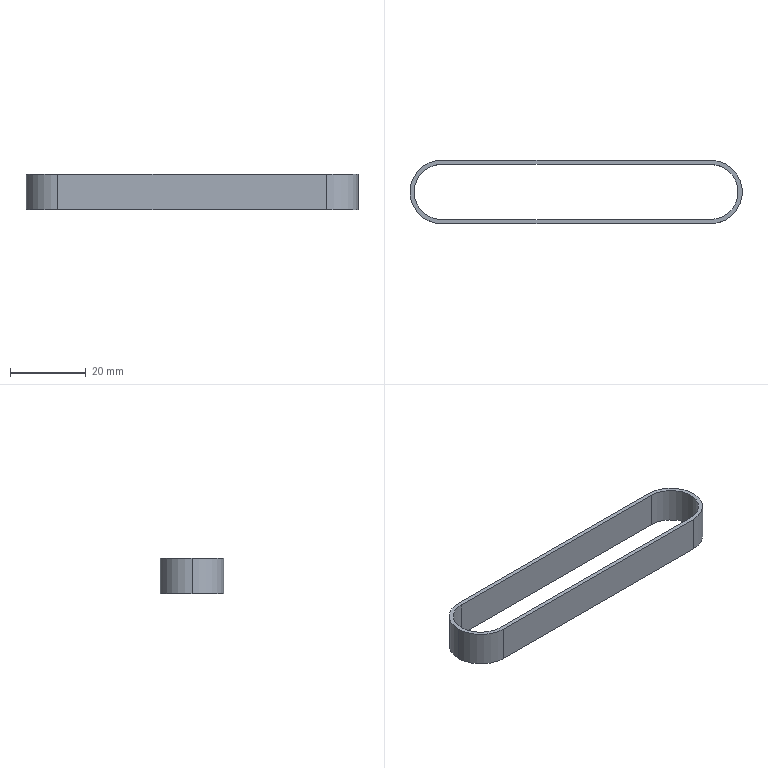Part | NX | features BREP 1 | 1 solid | 12 faces | box 87.76 x 16.76 x 9.5 mm | volume 1998 mm3 | plane 6 | cylinder 6 | commonest cylinder face diameters 14.56 x3 16.76 x3
STEP:
#1=CARTESIAN_POINT('',(-71.,-7.28,-4.75));
#2=VERTEX_POINT('',#1);
#3=CARTESIAN_POINT('',(0.,-7.28,-4.75));
#4=VERTEX_POINT('',#3);
#5=CARTESIAN_POINT('',(0.,-7.28,-4.75));
#6=DIRECTION('',(1.,0.,0.));
#7=VECTOR('',#6,1000.);
#8=LINE('',#5,#7);
#9=EDGE_CURVE('',#2,#4,#8,.T.);
#10=ORIENTED_EDGE('',*,*,#9,.F.);
#11=CARTESIAN_POINT('',(-71.,-7.28,4.75));
#12=VERTEX_POINT('',#11);
#13=CARTESIAN_POINT('',(-71.,-7.28,4.75));
#14=DIRECTION('',(0.,0.,-1.));
#15=VECTOR('',#14,1000.);
#16=LINE('',#13,#15);
#17=EDGE_CURVE('',#12,#2,#16,.T.);
#18=ORIENTED_EDGE('',*,*,#17,.F.);
#19=CARTESIAN_POINT('',(0.,-7.28,4.75));
#20=VERTEX_POINT('',#19);
#21=CARTESIAN_POINT('',(0.,-7.28,4.75));
#22=DIRECTION('',(1.,0.,0.));
#23=VECTOR('',#22,1000.);
#24=LINE('',#21,#23);
#25=EDGE_CURVE('',#12,#20,#24,.T.);
#26=ORIENTED_EDGE('',*,*,#25,.T.);
#27=CARTESIAN_POINT('',(0.,-7.28,4.75));
#28=DIRECTION('',(0.,0.,-1.));
#29=VECTOR('',#28,1000.);
#30=LINE('',#27,#29);
#31=EDGE_CURVE('',#20,#4,#30,.T.);
#32=ORIENTED_EDGE('',*,*,#31,.T.);
#33=EDGE_LOOP('',(#10,#18,#26,#32));
#34=FACE_BOUND('',#33,.T.);
#35=CARTESIAN_POINT('',(0.,-7.28,4.75));
#36=DIRECTION('',(0.,1.,0.));
#37=DIRECTION('',(0.,0.,1.));
#38=AXIS2_PLACEMENT_3D('',#35,#36,#37);
#39=PLANE('',#38);
#40=ADVANCED_FACE('',(#34),#39,.T.);
#41=CARTESIAN_POINT('',(-78.28,0.,4.75));
#42=VERTEX_POINT('',#41);
#43=CARTESIAN_POINT('',(-78.28,0.,-4.75));
#44=VERTEX_POINT('',#43);
#45=CARTESIAN_POINT('',(-78.28,0.,4.75));
#46=DIRECTION('',(0.,0.,-1.));
#47=VECTOR('',#46,1000.);
#48=LINE('',#45,#47);
#49=EDGE_CURVE('',#42,#44,#48,.T.);
#50=ORIENTED_EDGE('',*,*,#49,.F.);
#51=CARTESIAN_POINT('',(-71.,0.,4.75));
#52=DIRECTION('',(0.,0.,1.));
#53=DIRECTION('',(-1.,0.,0.));
#54=AXIS2_PLACEMENT_3D('',#51,#52,#53);
#55=CIRCLE('',#54,7.28);
#56=EDGE_CURVE('',#42,#12,#55,.T.);
#57=ORIENTED_EDGE('',*,*,#56,.T.);
#58=ORIENTED_EDGE('',*,*,#17,.T.);
#59=CARTESIAN_POINT('',(-71.,0.,-4.75));
#60=DIRECTION('',(0.,0.,1.));
#61=DIRECTION('',(-1.,0.,0.));
#62=AXIS2_PLACEMENT_3D('',#59,#60,#61);
#63=CIRCLE('',#62,7.28);
#64=EDGE_CURVE('',#44,#2,#63,.T.);
#65=ORIENTED_EDGE('',*,*,#64,.F.);
#66=EDGE_LOOP('',(#50,#57,#58,#65));
#67=FACE_BOUND('',#66,.T.);
#68=CARTESIAN_POINT('',(-71.,0.,4.75));
#69=DIRECTION('',(0.,0.,-1.));
#70=DIRECTION('',(-1.,0.,0.));
#71=AXIS2_PLACEMENT_3D('',#68,#69,#70);
#72=CYLINDRICAL_SURFACE('',#71,7.28);
#73=ADVANCED_FACE('',(#67),#72,.F.);
#74=CARTESIAN_POINT('',(0.,7.28,-4.75));
#75=VERTEX_POINT('',#74);
#76=CARTESIAN_POINT('',(-71.,7.28,-4.75));
#77=VERTEX_POINT('',#76);
#78=CARTESIAN_POINT('',(0.,7.28,-4.75));
#79=DIRECTION('',(-1.,0.,0.));
#80=VECTOR('',#79,1000.);
#81=LINE('',#78,#80);
#82=EDGE_CURVE('',#75,#77,#81,.T.);
#83=ORIENTED_EDGE('',*,*,#82,.F.);
#84=CARTESIAN_POINT('',(0.,7.28,4.75));
#85=VERTEX_POINT('',#84);
#86=CARTESIAN_POINT('',(0.,7.28,4.75));
#87=DIRECTION('',(0.,0.,-1.));
#88=VECTOR('',#87,1000.);
#89=LINE('',#86,#88);
#90=EDGE_CURVE('',#85,#75,#89,.T.);
#91=ORIENTED_EDGE('',*,*,#90,.F.);
#92=CARTESIAN_POINT('',(-71.,7.28,4.75));
#93=VERTEX_POINT('',#92);
#94=CARTESIAN_POINT('',(0.,7.28,4.75));
#95=DIRECTION('',(-1.,0.,0.));
#96=VECTOR('',#95,1000.);
#97=LINE('',#94,#96);
#98=EDGE_CURVE('',#85,#93,#97,.T.);
#99=ORIENTED_EDGE('',*,*,#98,.T.);
#100=CARTESIAN_POINT('',(-71.,7.28,4.75));
#101=DIRECTION('',(0.,0.,-1.));
#102=VECTOR('',#101,1000.);
#103=LINE('',#100,#102);
#104=EDGE_CURVE('',#93,#77,#103,.T.);
#105=ORIENTED_EDGE('',*,*,#104,.T.);
#106=EDGE_LOOP('',(#83,#91,#99,#105));
#107=FACE_BOUND('',#106,.T.);
#108=CARTESIAN_POINT('',(0.,7.28,4.75));
#109=DIRECTION('',(0.,-1.,0.));
#110=DIRECTION('',(0.,0.,-1.));
#111=AXIS2_PLACEMENT_3D('',#108,#109,#110);
#112=PLANE('',#111);
#113=ADVANCED_FACE('',(#107),#112,.T.);
#114=CARTESIAN_POINT('',(0.,0.,-4.75));
#115=DIRECTION('',(0.,0.,1.));
#116=DIRECTION('',(-1.,0.,0.));
#117=AXIS2_PLACEMENT_3D('',#114,#115,#116);
#118=CIRCLE('',#117,7.28);
#119=EDGE_CURVE('',#4,#75,#118,.T.);
#120=ORIENTED_EDGE('',*,*,#119,.F.);
#121=ORIENTED_EDGE('',*,*,#31,.F.);
#122=CARTESIAN_POINT('',(0.,0.,4.75));
#123=DIRECTION('',(0.,0.,1.));
#124=DIRECTION('',(-1.,0.,0.));
#125=AXIS2_PLACEMENT_3D('',#122,#123,#124);
#126=CIRCLE('',#125,7.28);
#127=EDGE_CURVE('',#20,#85,#126,.T.);
#128=ORIENTED_EDGE('',*,*,#127,.T.);
#129=ORIENTED_EDGE('',*,*,#90,.T.);
#130=EDGE_LOOP('',(#120,#121,#128,#129));
#131=FACE_BOUND('',#130,.T.);
#132=CARTESIAN_POINT('',(0.,0.,4.75));
#133=DIRECTION('',(0.,0.,-1.));
#134=DIRECTION('',(-1.,0.,0.));
#135=AXIS2_PLACEMENT_3D('',#132,#133,#134);
#136=CYLINDRICAL_SURFACE('',#135,7.28);
#137=ADVANCED_FACE('',(#131),#136,.F.);
#138=CARTESIAN_POINT('',(-71.,-8.38,-4.75));
#139=VERTEX_POINT('',#138);
#140=CARTESIAN_POINT('',(0.,-8.38,-4.75));
#141=VERTEX_POINT('',#140);
#142=CARTESIAN_POINT('',(0.,-8.38,-4.75));
#143=DIRECTION('',(1.,0.,0.));
#144=VECTOR('',#143,1000.);
#145=LINE('',#142,#144);
#146=EDGE_CURVE('',#139,#141,#145,.T.);
#147=ORIENTED_EDGE('',*,*,#146,.T.);
#148=CARTESIAN_POINT('',(0.,-8.38,4.75));
#149=VERTEX_POINT('',#148);
#150=CARTESIAN_POINT('',(0.,-8.38,4.75));
#151=DIRECTION('',(0.,0.,-1.));
#152=VECTOR('',#151,1000.);
#153=LINE('',#150,#152);
#154=EDGE_CURVE('',#149,#141,#153,.T.);
#155=ORIENTED_EDGE('',*,*,#154,.F.);
#156=CARTESIAN_POINT('',(-71.,-8.38,4.75));
#157=VERTEX_POINT('',#156);
#158=CARTESIAN_POINT('',(0.,-8.38,4.75));
#159=DIRECTION('',(1.,0.,0.));
#160=VECTOR('',#159,1000.);
#161=LINE('',#158,#160);
#162=EDGE_CURVE('',#157,#149,#161,.T.);
#163=ORIENTED_EDGE('',*,*,#162,.F.);
#164=CARTESIAN_POINT('',(-71.,-8.38,4.75));
#165=DIRECTION('',(0.,0.,-1.));
#166=VECTOR('',#165,1000.);
#167=LINE('',#164,#166);
#168=EDGE_CURVE('',#157,#139,#167,.T.);
#169=ORIENTED_EDGE('',*,*,#168,.T.);
#170=EDGE_LOOP('',(#147,#155,#163,#169));
#171=FACE_BOUND('',#170,.T.);
#172=CARTESIAN_POINT('',(0.,-8.38,4.75));
#173=DIRECTION('',(0.,1.,0.));
#174=DIRECTION('',(0.,0.,1.));
#175=AXIS2_PLACEMENT_3D('',#172,#173,#174);
#176=PLANE('',#175);
#177=ADVANCED_FACE('',(#171),#176,.F.);
#178=CARTESIAN_POINT('',(-79.38,0.,4.75));
#179=VERTEX_POINT('',#178);
#180=CARTESIAN_POINT('',(-79.38,0.,-4.75));
#181=VERTEX_POINT('',#180);
#182=CARTESIAN_POINT('',(-79.38,0.,4.75));
#183=DIRECTION('',(0.,0.,-1.));
#184=VECTOR('',#183,1000.);
#185=LINE('',#182,#184);
#186=EDGE_CURVE('',#179,#181,#185,.T.);
#187=ORIENTED_EDGE('',*,*,#186,.F.);
#188=CARTESIAN_POINT('',(-71.,8.38,4.75));
#189=VERTEX_POINT('',#188);
#190=CARTESIAN_POINT('',(-71.,0.,4.75));
#191=DIRECTION('',(0.,0.,1.));
#192=DIRECTION('',(-1.,0.,0.));
#193=AXIS2_PLACEMENT_3D('',#190,#191,#192);
#194=CIRCLE('',#193,8.38);
#195=EDGE_CURVE('',#189,#179,#194,.T.);
#196=ORIENTED_EDGE('',*,*,#195,.F.);
#197=CARTESIAN_POINT('',(-71.,8.38,-4.75));
#198=VERTEX_POINT('',#197);
#199=CARTESIAN_POINT('',(-71.,8.38,4.75));
#200=DIRECTION('',(0.,0.,-1.));
#201=VECTOR('',#200,1000.);
#202=LINE('',#199,#201);
#203=EDGE_CURVE('',#189,#198,#202,.T.);
#204=ORIENTED_EDGE('',*,*,#203,.T.);
#205=CARTESIAN_POINT('',(-71.,0.,-4.75));
#206=DIRECTION('',(0.,0.,1.));
#207=DIRECTION('',(-1.,0.,0.));
#208=AXIS2_PLACEMENT_3D('',#205,#206,#207);
#209=CIRCLE('',#208,8.38);
#210=EDGE_CURVE('',#198,#181,#209,.T.);
#211=ORIENTED_EDGE('',*,*,#210,.T.);
#212=EDGE_LOOP('',(#187,#196,#204,#211));
#213=FACE_BOUND('',#212,.T.);
#214=CARTESIAN_POINT('',(-71.,0.,4.75));
#215=DIRECTION('',(0.,0.,-1.));
#216=DIRECTION('',(-1.,0.,0.));
#217=AXIS2_PLACEMENT_3D('',#214,#215,#216);
#218=CYLINDRICAL_SURFACE('',#217,8.38);
#219=ADVANCED_FACE('',(#213),#218,.T.);
#220=CARTESIAN_POINT('',(0.,8.38,-4.75));
#221=VERTEX_POINT('',#220);
#222=CARTESIAN_POINT('',(0.,8.38,-4.75));
#223=DIRECTION('',(-1.,0.,0.));
#224=VECTOR('',#223,1000.);
#225=LINE('',#222,#224);
#226=EDGE_CURVE('',#221,#198,#225,.T.);
#227=ORIENTED_EDGE('',*,*,#226,.T.);
#228=ORIENTED_EDGE('',*,*,#203,.F.);
#229=CARTESIAN_POINT('',(0.,8.38,4.75));
#230=VERTEX_POINT('',#229);
#231=CARTESIAN_POINT('',(0.,8.38,4.75));
#232=DIRECTION('',(-1.,0.,0.));
#233=VECTOR('',#232,1000.);
#234=LINE('',#231,#233);
#235=EDGE_CURVE('',#230,#189,#234,.T.);
#236=ORIENTED_EDGE('',*,*,#235,.F.);
#237=CARTESIAN_POINT('',(0.,8.38,4.75));
#238=DIRECTION('',(0.,0.,-1.));
#239=VECTOR('',#238,1000.);
#240=LINE('',#237,#239);
#241=EDGE_CURVE('',#230,#221,#240,.T.);
#242=ORIENTED_EDGE('',*,*,#241,.T.);
#243=EDGE_LOOP('',(#227,#228,#236,#242));
#244=FACE_BOUND('',#243,.T.);
#245=CARTESIAN_POINT('',(0.,8.38,4.75));
#246=DIRECTION('',(0.,-1.,0.));
#247=DIRECTION('',(0.,0.,-1.));
#248=AXIS2_PLACEMENT_3D('',#245,#246,#247);
#249=PLANE('',#248);
#250=ADVANCED_FACE('',(#244),#249,.F.);
#251=CARTESIAN_POINT('',(0.,0.,-4.75));
#252=DIRECTION('',(0.,0.,1.));
#253=DIRECTION('',(-1.,0.,0.));
#254=AXIS2_PLACEMENT_3D('',#251,#252,#253);
#255=CIRCLE('',#254,8.38);
#256=EDGE_CURVE('',#141,#221,#255,.T.);
#257=ORIENTED_EDGE('',*,*,#256,.T.);
#258=ORIENTED_EDGE('',*,*,#241,.F.);
#259=CARTESIAN_POINT('',(0.,0.,4.75));
#260=DIRECTION('',(0.,0.,1.));
#261=DIRECTION('',(-1.,0.,0.));
#262=AXIS2_PLACEMENT_3D('',#259,#260,#261);
#263=CIRCLE('',#262,8.38);
#264=EDGE_CURVE('',#149,#230,#263,.T.);
#265=ORIENTED_EDGE('',*,*,#264,.F.);
#266=ORIENTED_EDGE('',*,*,#154,.T.);
#267=EDGE_LOOP('',(#257,#258,#265,#266));
#268=FACE_BOUND('',#267,.T.);
#269=CARTESIAN_POINT('',(0.,0.,4.75));
#270=DIRECTION('',(0.,0.,-1.));
#271=DIRECTION('',(-1.,0.,0.));
#272=AXIS2_PLACEMENT_3D('',#269,#270,#271);
#273=CYLINDRICAL_SURFACE('',#272,8.38);
#274=ADVANCED_FACE('',(#268),#273,.T.);
#275=ORIENTED_EDGE('',*,*,#9,.T.);
#276=ORIENTED_EDGE('',*,*,#119,.T.);
#277=ORIENTED_EDGE('',*,*,#82,.T.);
#278=CARTESIAN_POINT('',(-71.,0.,-4.75));
#279=DIRECTION('',(0.,0.,1.));
#280=DIRECTION('',(-1.,0.,0.));
#281=AXIS2_PLACEMENT_3D('',#278,#279,#280);
#282=CIRCLE('',#281,7.28);
#283=EDGE_CURVE('',#77,#44,#282,.T.);
#284=ORIENTED_EDGE('',*,*,#283,.T.);
#285=ORIENTED_EDGE('',*,*,#64,.T.);
#286=EDGE_LOOP('',(#275,#276,#277,#284,#285));
#287=FACE_BOUND('',#286,.T.);
#288=ORIENTED_EDGE('',*,*,#256,.F.);
#289=ORIENTED_EDGE('',*,*,#146,.F.);
#290=CARTESIAN_POINT('',(-71.,0.,-4.75));
#291=DIRECTION('',(0.,0.,1.));
#292=DIRECTION('',(-1.,0.,0.));
#293=AXIS2_PLACEMENT_3D('',#290,#291,#292);
#294=CIRCLE('',#293,8.38);
#295=EDGE_CURVE('',#181,#139,#294,.T.);
#296=ORIENTED_EDGE('',*,*,#295,.F.);
#297=ORIENTED_EDGE('',*,*,#210,.F.);
#298=ORIENTED_EDGE('',*,*,#226,.F.);
#299=EDGE_LOOP('',(#288,#289,#296,#297,#298));
#300=FACE_BOUND('',#299,.T.);
#301=CARTESIAN_POINT('',(0.,0.,-4.75));
#302=DIRECTION('',(0.,0.,-1.));
#303=DIRECTION('',(-1.,0.,0.));
#304=AXIS2_PLACEMENT_3D('',#301,#302,#303);
#305=PLANE('',#304);
#306=ADVANCED_FACE('',(#287,#300),#305,.T.);
#307=ORIENTED_EDGE('',*,*,#127,.F.);
#308=ORIENTED_EDGE('',*,*,#25,.F.);
#309=ORIENTED_EDGE('',*,*,#56,.F.);
#310=CARTESIAN_POINT('',(-71.,0.,4.75));
#311=DIRECTION('',(0.,0.,1.));
#312=DIRECTION('',(-1.,0.,0.));
#313=AXIS2_PLACEMENT_3D('',#310,#311,#312);
#314=CIRCLE('',#313,7.28);
#315=EDGE_CURVE('',#93,#42,#314,.T.);
#316=ORIENTED_EDGE('',*,*,#315,.F.);
#317=ORIENTED_EDGE('',*,*,#98,.F.);
#318=EDGE_LOOP('',(#307,#308,#309,#316,#317));
#319=FACE_BOUND('',#318,.T.);
#320=ORIENTED_EDGE('',*,*,#264,.T.);
#321=ORIENTED_EDGE('',*,*,#235,.T.);
#322=ORIENTED_EDGE('',*,*,#195,.T.);
#323=CARTESIAN_POINT('',(-71.,0.,4.75));
#324=DIRECTION('',(0.,0.,1.));
#325=DIRECTION('',(-1.,0.,0.));
#326=AXIS2_PLACEMENT_3D('',#323,#324,#325);
#327=CIRCLE('',#326,8.38);
#328=EDGE_CURVE('',#179,#157,#327,.T.);
#329=ORIENTED_EDGE('',*,*,#328,.T.);
#330=ORIENTED_EDGE('',*,*,#162,.T.);
#331=EDGE_LOOP('',(#320,#321,#322,#329,#330));
#332=FACE_BOUND('',#331,.T.);
#333=CARTESIAN_POINT('',(0.,0.,4.75));
#334=DIRECTION('',(0.,0.,-1.));
#335=DIRECTION('',(-1.,0.,0.));
#336=AXIS2_PLACEMENT_3D('',#333,#334,#335);
#337=PLANE('',#336);
#338=ADVANCED_FACE('',(#319,#332),#337,.F.);
#339=ORIENTED_EDGE('',*,*,#328,.F.);
#340=ORIENTED_EDGE('',*,*,#186,.T.);
#341=ORIENTED_EDGE('',*,*,#295,.T.);
#342=ORIENTED_EDGE('',*,*,#168,.F.);
#343=EDGE_LOOP('',(#339,#340,#341,#342));
#344=FACE_BOUND('',#343,.T.);
#345=CARTESIAN_POINT('',(-71.,0.,4.75));
#346=DIRECTION('',(0.,0.,-1.));
#347=DIRECTION('',(-1.,0.,0.));
#348=AXIS2_PLACEMENT_3D('',#345,#346,#347);
#349=CYLINDRICAL_SURFACE('',#348,8.38);
#350=ADVANCED_FACE('',(#344),#349,.T.);
#351=ORIENTED_EDGE('',*,*,#315,.T.);
#352=ORIENTED_EDGE('',*,*,#49,.T.);
#353=ORIENTED_EDGE('',*,*,#283,.F.);
#354=ORIENTED_EDGE('',*,*,#104,.F.);
#355=EDGE_LOOP('',(#351,#352,#353,#354));
#356=FACE_BOUND('',#355,.T.);
#357=CARTESIAN_POINT('',(-71.,0.,4.75));
#358=DIRECTION('',(0.,0.,-1.));
#359=DIRECTION('',(-1.,0.,0.));
#360=AXIS2_PLACEMENT_3D('',#357,#358,#359);
#361=CYLINDRICAL_SURFACE('',#360,7.28);
#362=ADVANCED_FACE('',(#356),#361,.F.);
#363=CLOSED_SHELL('',(#40,#73,#113,#137,#177,#219,#250,#274,#306,#338,#350,#362));
#364=MANIFOLD_SOLID_BREP('',#363);
#365=(LENGTH_UNIT()NAMED_UNIT(*)SI_UNIT(.MILLI.,.METRE.));
#366=UNCERTAINTY_MEASURE_WITH_UNIT(LENGTH_MEASURE(0.00001),#365,'','');
#367=(NAMED_UNIT(*)PLANE_ANGLE_UNIT()SI_UNIT($,.RADIAN.));
#368=(NAMED_UNIT(*)SI_UNIT($,.STERADIAN.)SOLID_ANGLE_UNIT());
#369=(GEOMETRIC_REPRESENTATION_CONTEXT(3)GLOBAL_UNCERTAINTY_ASSIGNED_CONTEXT((#366))GLOBAL_UNIT_ASSIGNED_CONTEXT((#365,#367,#368))REPRESENTATION_CONTEXT('',''));
#370=ADVANCED_BREP_SHAPE_REPRESENTATION('',(#364),#369);